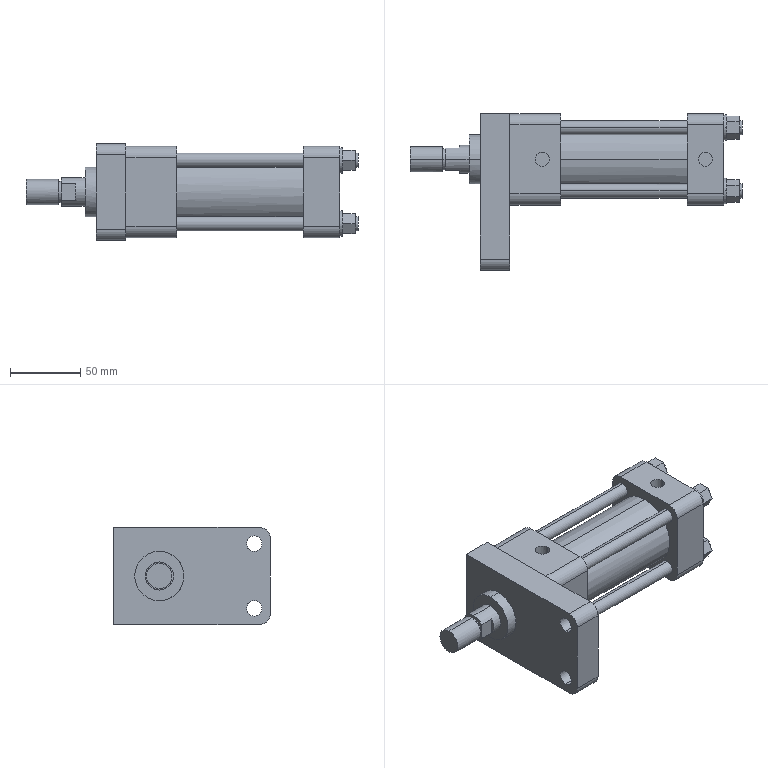Part | Creo | 1 solid | 114 faces | box 236 x 111.5 x 69 mm | volume 643114 mm3 | plane 62 | cylinder 52 | commonest cylinder face diameters 10 x20 16 x10 18 x10 11 x4 15 x2 20 x2